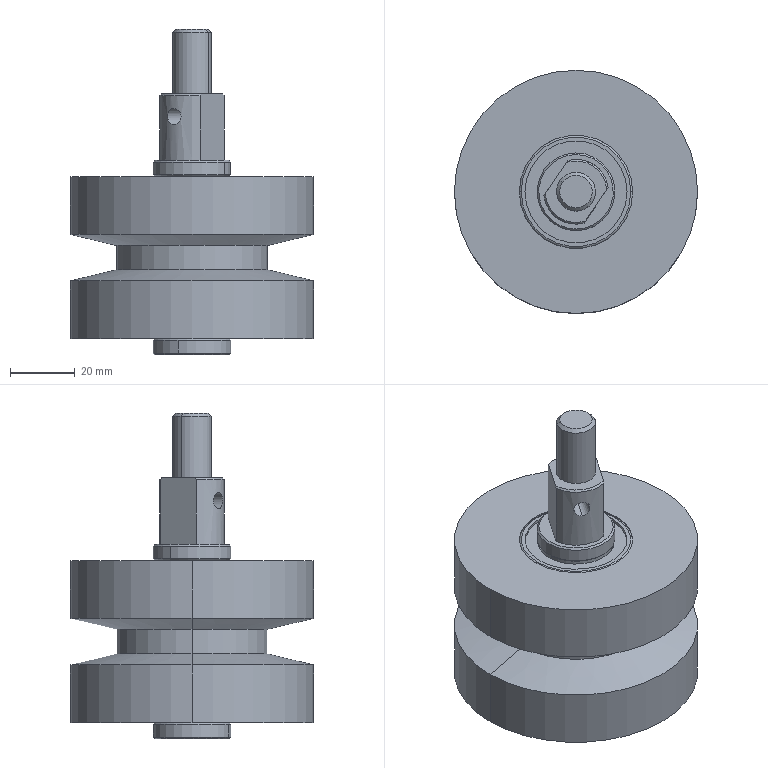Part | SolidWorks | 5 solids | 351 faces | box 75 x 75 x 100.5 mm | volume 180032 mm3 | sphere 128 | cylinder 76 | torus 64 | plane 61 | cone 22 | commonest cylinder face diameters 31.5 x16 21.6 x8 23.564 x8 35 x8 15 x6 5 x4